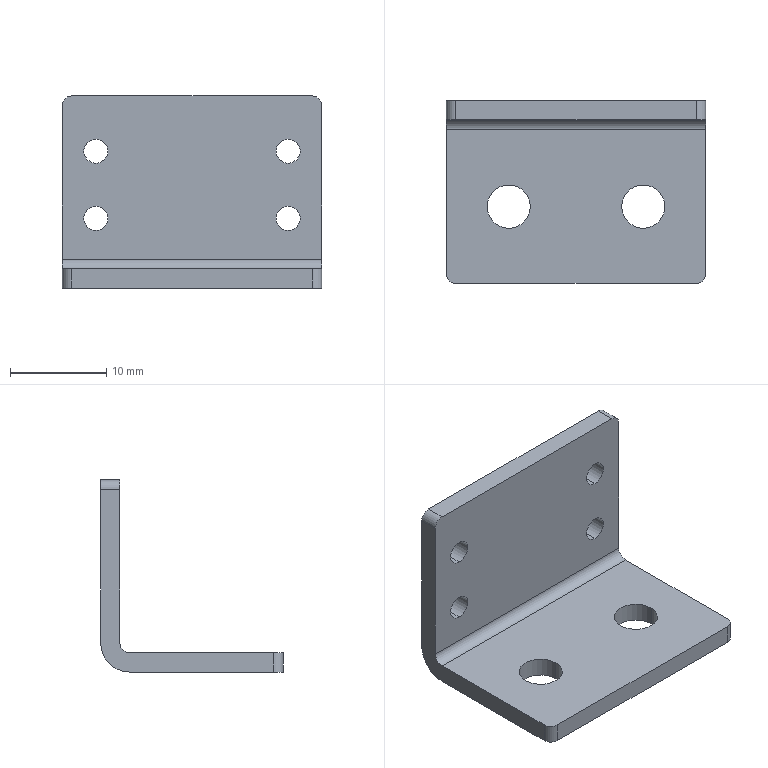Part | SolidWorks | features BaseBody 1 | 1 solid | 26 faces | box 27 x 19 x 20 mm | volume 1847 mm3 | cylinder 18 | plane 8 | commonest cylinder face diameters 2.5 x8 2 x5 4.5 x4 6 x1
STEP:
#1=CARTESIAN_POINT('',(10.,17.,3.));
#2=VERTEX_POINT('',#1);
#3=CARTESIAN_POINT('',(10.,17.,5.5));
#4=VERTEX_POINT('',#3);
#5=CARTESIAN_POINT('',(10.,17.,4.25));
#6=DIRECTION('',(0.,1.,0.));
#7=DIRECTION('',(0.,0.,1.));
#8=AXIS2_PLACEMENT_3D('',#5,#6,#7);
#9=CIRCLE('',#8,1.25);
#10=EDGE_CURVE('',#2,#4,#9,.T.);
#11=ORIENTED_EDGE('',*,*,#10,.F.);
#12=CARTESIAN_POINT('',(10.,19.,3.));
#13=VERTEX_POINT('',#12);
#14=CARTESIAN_POINT('',(10.,19.,3.));
#15=DIRECTION('',(0.,1.,0.));
#16=VECTOR('',#15,1000.);
#17=LINE('',#14,#16);
#18=EDGE_CURVE('',#2,#13,#17,.T.);
#19=ORIENTED_EDGE('',*,*,#18,.T.);
#20=CARTESIAN_POINT('',(10.,19.,5.5));
#21=VERTEX_POINT('',#20);
#22=CARTESIAN_POINT('',(10.,19.,4.25));
#23=DIRECTION('',(0.,-1.,0.));
#24=DIRECTION('',(0.,0.,1.));
#25=AXIS2_PLACEMENT_3D('',#22,#23,#24);
#26=CIRCLE('',#25,1.25);
#27=EDGE_CURVE('',#21,#13,#26,.T.);
#28=ORIENTED_EDGE('',*,*,#27,.F.);
#29=CARTESIAN_POINT('',(10.,19.,5.5));
#30=DIRECTION('',(0.,1.,0.));
#31=VECTOR('',#30,1000.);
#32=LINE('',#29,#31);
#33=EDGE_CURVE('',#4,#21,#32,.T.);
#34=ORIENTED_EDGE('',*,*,#33,.F.);
#35=EDGE_LOOP('',(#11,#19,#28,#34));
#36=FACE_OUTER_BOUND('',#35,.T.);
#37=CARTESIAN_POINT('',(10.,19.,4.25));
#38=DIRECTION('',(0.,1.,0.));
#39=DIRECTION('',(0.,0.,1.));
#40=AXIS2_PLACEMENT_3D('',#37,#38,#39);
#41=CYLINDRICAL_SURFACE('',#40,1.25);
#42=ADVANCED_FACE('',(#36),#41,.F.);
#43=CARTESIAN_POINT('',(10.,17.,-4.));
#44=VERTEX_POINT('',#43);
#45=CARTESIAN_POINT('',(10.,17.,-1.5));
#46=VERTEX_POINT('',#45);
#47=CARTESIAN_POINT('',(10.,17.,-2.75));
#48=DIRECTION('',(0.,1.,0.));
#49=DIRECTION('',(0.,0.,1.));
#50=AXIS2_PLACEMENT_3D('',#47,#48,#49);
#51=CIRCLE('',#50,1.25);
#52=EDGE_CURVE('',#44,#46,#51,.T.);
#53=ORIENTED_EDGE('',*,*,#52,.F.);
#54=CARTESIAN_POINT('',(10.,19.,-4.));
#55=VERTEX_POINT('',#54);
#56=CARTESIAN_POINT('',(10.,19.,-4.));
#57=DIRECTION('',(0.,1.,0.));
#58=VECTOR('',#57,1000.);
#59=LINE('',#56,#58);
#60=EDGE_CURVE('',#44,#55,#59,.T.);
#61=ORIENTED_EDGE('',*,*,#60,.T.);
#62=CARTESIAN_POINT('',(10.,19.,-1.5));
#63=VERTEX_POINT('',#62);
#64=CARTESIAN_POINT('',(10.,19.,-2.75));
#65=DIRECTION('',(0.,-1.,0.));
#66=DIRECTION('',(0.,0.,1.));
#67=AXIS2_PLACEMENT_3D('',#64,#65,#66);
#68=CIRCLE('',#67,1.25);
#69=EDGE_CURVE('',#63,#55,#68,.T.);
#70=ORIENTED_EDGE('',*,*,#69,.F.);
#71=CARTESIAN_POINT('',(10.,19.,-1.5));
#72=DIRECTION('',(0.,1.,0.));
#73=VECTOR('',#72,1000.);
#74=LINE('',#71,#73);
#75=EDGE_CURVE('',#46,#63,#74,.T.);
#76=ORIENTED_EDGE('',*,*,#75,.F.);
#77=EDGE_LOOP('',(#53,#61,#70,#76));
#78=FACE_OUTER_BOUND('',#77,.T.);
#79=CARTESIAN_POINT('',(10.,19.,-2.75));
#80=DIRECTION('',(0.,1.,0.));
#81=DIRECTION('',(0.,0.,1.));
#82=AXIS2_PLACEMENT_3D('',#79,#80,#81);
#83=CYLINDRICAL_SURFACE('',#82,1.25);
#84=ADVANCED_FACE('',(#78),#83,.F.);
#85=CARTESIAN_POINT('',(-10.,17.,-4.));
#86=VERTEX_POINT('',#85);
#87=CARTESIAN_POINT('',(-10.,17.,-1.5));
#88=VERTEX_POINT('',#87);
#89=CARTESIAN_POINT('',(-10.,17.,-2.75));
#90=DIRECTION('',(0.,1.,0.));
#91=DIRECTION('',(0.,0.,1.));
#92=AXIS2_PLACEMENT_3D('',#89,#90,#91);
#93=CIRCLE('',#92,1.25);
#94=EDGE_CURVE('',#86,#88,#93,.T.);
#95=ORIENTED_EDGE('',*,*,#94,.F.);
#96=CARTESIAN_POINT('',(-10.,19.,-4.));
#97=VERTEX_POINT('',#96);
#98=CARTESIAN_POINT('',(-10.,19.,-4.));
#99=DIRECTION('',(0.,1.,0.));
#100=VECTOR('',#99,1000.);
#101=LINE('',#98,#100);
#102=EDGE_CURVE('',#86,#97,#101,.T.);
#103=ORIENTED_EDGE('',*,*,#102,.T.);
#104=CARTESIAN_POINT('',(-10.,19.,-1.5));
#105=VERTEX_POINT('',#104);
#106=CARTESIAN_POINT('',(-10.,19.,-2.75));
#107=DIRECTION('',(0.,-1.,0.));
#108=DIRECTION('',(0.,0.,1.));
#109=AXIS2_PLACEMENT_3D('',#106,#107,#108);
#110=CIRCLE('',#109,1.25);
#111=EDGE_CURVE('',#105,#97,#110,.T.);
#112=ORIENTED_EDGE('',*,*,#111,.F.);
#113=CARTESIAN_POINT('',(-10.,19.,-1.5));
#114=DIRECTION('',(0.,1.,0.));
#115=VECTOR('',#114,1000.);
#116=LINE('',#113,#115);
#117=EDGE_CURVE('',#88,#105,#116,.T.);
#118=ORIENTED_EDGE('',*,*,#117,.F.);
#119=EDGE_LOOP('',(#95,#103,#112,#118));
#120=FACE_OUTER_BOUND('',#119,.T.);
#121=CARTESIAN_POINT('',(-10.,19.,-2.75));
#122=DIRECTION('',(0.,1.,0.));
#123=DIRECTION('',(0.,0.,1.));
#124=AXIS2_PLACEMENT_3D('',#121,#122,#123);
#125=CYLINDRICAL_SURFACE('',#124,1.25);
#126=ADVANCED_FACE('',(#120),#125,.F.);
#127=CARTESIAN_POINT('',(-10.,17.,3.));
#128=VERTEX_POINT('',#127);
#129=CARTESIAN_POINT('',(-10.,17.,5.5));
#130=VERTEX_POINT('',#129);
#131=CARTESIAN_POINT('',(-10.,17.,4.25));
#132=DIRECTION('',(0.,1.,0.));
#133=DIRECTION('',(0.,0.,1.));
#134=AXIS2_PLACEMENT_3D('',#131,#132,#133);
#135=CIRCLE('',#134,1.25);
#136=EDGE_CURVE('',#128,#130,#135,.T.);
#137=ORIENTED_EDGE('',*,*,#136,.F.);
#138=CARTESIAN_POINT('',(-10.,19.,3.));
#139=VERTEX_POINT('',#138);
#140=CARTESIAN_POINT('',(-10.,19.,3.));
#141=DIRECTION('',(0.,1.,0.));
#142=VECTOR('',#141,1000.);
#143=LINE('',#140,#142);
#144=EDGE_CURVE('',#128,#139,#143,.T.);
#145=ORIENTED_EDGE('',*,*,#144,.T.);
#146=CARTESIAN_POINT('',(-10.,19.,5.5));
#147=VERTEX_POINT('',#146);
#148=CARTESIAN_POINT('',(-10.,19.,4.25));
#149=DIRECTION('',(0.,-1.,0.));
#150=DIRECTION('',(0.,0.,1.));
#151=AXIS2_PLACEMENT_3D('',#148,#149,#150);
#152=CIRCLE('',#151,1.25);
#153=EDGE_CURVE('',#147,#139,#152,.T.);
#154=ORIENTED_EDGE('',*,*,#153,.F.);
#155=CARTESIAN_POINT('',(-10.,19.,5.5));
#156=DIRECTION('',(0.,1.,0.));
#157=VECTOR('',#156,1000.);
#158=LINE('',#155,#157);
#159=EDGE_CURVE('',#130,#147,#158,.T.);
#160=ORIENTED_EDGE('',*,*,#159,.F.);
#161=EDGE_LOOP('',(#137,#145,#154,#160));
#162=FACE_OUTER_BOUND('',#161,.T.);
#163=CARTESIAN_POINT('',(-10.,19.,4.25));
#164=DIRECTION('',(0.,1.,0.));
#165=DIRECTION('',(0.,0.,1.));
#166=AXIS2_PLACEMENT_3D('',#163,#164,#165);
#167=CYLINDRICAL_SURFACE('',#166,1.25);
#168=ADVANCED_FACE('',(#162),#167,.F.);
#169=CARTESIAN_POINT('',(9.25,8.,-8.));
#170=VERTEX_POINT('',#169);
#171=CARTESIAN_POINT('',(4.75,8.,-8.));
#172=VERTEX_POINT('',#171);
#173=CARTESIAN_POINT('',(7.,8.,-8.));
#174=DIRECTION('',(0.,0.,-1.));
#175=DIRECTION('',(-1.,0.,0.));
#176=AXIS2_PLACEMENT_3D('',#173,#174,#175);
#177=CIRCLE('',#176,2.25);
#178=EDGE_CURVE('',#170,#172,#177,.T.);
#179=ORIENTED_EDGE('',*,*,#178,.F.);
#180=CARTESIAN_POINT('',(9.25,8.,-10.));
#181=VERTEX_POINT('',#180);
#182=CARTESIAN_POINT('',(9.25,8.,-10.));
#183=DIRECTION('',(0.,0.,-1.));
#184=VECTOR('',#183,1000.);
#185=LINE('',#182,#184);
#186=EDGE_CURVE('',#170,#181,#185,.T.);
#187=ORIENTED_EDGE('',*,*,#186,.T.);
#188=CARTESIAN_POINT('',(4.75,8.,-10.));
#189=VERTEX_POINT('',#188);
#190=CARTESIAN_POINT('',(7.,8.,-10.));
#191=DIRECTION('',(0.,0.,-1.));
#192=DIRECTION('',(-1.,0.,0.));
#193=AXIS2_PLACEMENT_3D('',#190,#191,#192);
#194=CIRCLE('',#193,2.25);
#195=EDGE_CURVE('',#181,#189,#194,.T.);
#196=ORIENTED_EDGE('',*,*,#195,.T.);
#197=CARTESIAN_POINT('',(4.75,8.,-10.));
#198=DIRECTION('',(0.,0.,-1.));
#199=VECTOR('',#198,1000.);
#200=LINE('',#197,#199);
#201=EDGE_CURVE('',#172,#189,#200,.T.);
#202=ORIENTED_EDGE('',*,*,#201,.F.);
#203=EDGE_LOOP('',(#179,#187,#196,#202));
#204=FACE_OUTER_BOUND('',#203,.T.);
#205=CARTESIAN_POINT('',(7.,8.,-10.));
#206=DIRECTION('',(0.,0.,-1.));
#207=DIRECTION('',(-1.,0.,0.));
#208=AXIS2_PLACEMENT_3D('',#205,#206,#207);
#209=CYLINDRICAL_SURFACE('',#208,2.25);
#210=ADVANCED_FACE('',(#204),#209,.F.);
#211=CARTESIAN_POINT('',(-4.75,8.,-8.));
#212=VERTEX_POINT('',#211);
#213=CARTESIAN_POINT('',(-9.25,8.,-8.));
#214=VERTEX_POINT('',#213);
#215=CARTESIAN_POINT('',(-7.,8.,-8.));
#216=DIRECTION('',(0.,0.,-1.));
#217=DIRECTION('',(-1.,0.,0.));
#218=AXIS2_PLACEMENT_3D('',#215,#216,#217);
#219=CIRCLE('',#218,2.25);
#220=EDGE_CURVE('',#212,#214,#219,.T.);
#221=ORIENTED_EDGE('',*,*,#220,.F.);
#222=CARTESIAN_POINT('',(-4.75,8.,-10.));
#223=VERTEX_POINT('',#222);
#224=CARTESIAN_POINT('',(-4.75,8.,-10.));
#225=DIRECTION('',(0.,0.,-1.));
#226=VECTOR('',#225,1000.);
#227=LINE('',#224,#226);
#228=EDGE_CURVE('',#212,#223,#227,.T.);
#229=ORIENTED_EDGE('',*,*,#228,.T.);
#230=CARTESIAN_POINT('',(-9.25,8.,-10.));
#231=VERTEX_POINT('',#230);
#232=CARTESIAN_POINT('',(-7.,8.,-10.));
#233=DIRECTION('',(0.,0.,-1.));
#234=DIRECTION('',(-1.,0.,0.));
#235=AXIS2_PLACEMENT_3D('',#232,#233,#234);
#236=CIRCLE('',#235,2.25);
#237=EDGE_CURVE('',#223,#231,#236,.T.);
#238=ORIENTED_EDGE('',*,*,#237,.T.);
#239=CARTESIAN_POINT('',(-9.25,8.,-10.));
#240=DIRECTION('',(0.,0.,-1.));
#241=VECTOR('',#240,1000.);
#242=LINE('',#239,#241);
#243=EDGE_CURVE('',#214,#231,#242,.T.);
#244=ORIENTED_EDGE('',*,*,#243,.F.);
#245=EDGE_LOOP('',(#221,#229,#238,#244));
#246=FACE_OUTER_BOUND('',#245,.T.);
#247=CARTESIAN_POINT('',(-7.,8.,-10.));
#248=DIRECTION('',(0.,0.,-1.));
#249=DIRECTION('',(-1.,0.,0.));
#250=AXIS2_PLACEMENT_3D('',#247,#248,#249);
#251=CYLINDRICAL_SURFACE('',#250,2.25);
#252=ADVANCED_FACE('',(#246),#251,.F.);
#253=ORIENTED_EDGE('',*,*,#27,.T.);
#254=CARTESIAN_POINT('',(10.,19.,4.25));
#255=DIRECTION('',(0.,-1.,0.));
#256=DIRECTION('',(0.,0.,1.));
#257=AXIS2_PLACEMENT_3D('',#254,#255,#256);
#258=CIRCLE('',#257,1.25);
#259=EDGE_CURVE('',#13,#21,#258,.T.);
#260=ORIENTED_EDGE('',*,*,#259,.T.);
#261=EDGE_LOOP('',(#253,#260));
#262=FACE_BOUND('',#261,.T.);
#263=ORIENTED_EDGE('',*,*,#69,.T.);
#264=CARTESIAN_POINT('',(10.,19.,-2.75));
#265=DIRECTION('',(0.,-1.,0.));
#266=DIRECTION('',(0.,0.,1.));
#267=AXIS2_PLACEMENT_3D('',#264,#265,#266);
#268=CIRCLE('',#267,1.25);
#269=EDGE_CURVE('',#55,#63,#268,.T.);
#270=ORIENTED_EDGE('',*,*,#269,.T.);
#271=EDGE_LOOP('',(#263,#270));
#272=FACE_BOUND('',#271,.T.);
#273=ORIENTED_EDGE('',*,*,#111,.T.);
#274=CARTESIAN_POINT('',(-10.,19.,-2.75));
#275=DIRECTION('',(0.,-1.,0.));
#276=DIRECTION('',(0.,0.,1.));
#277=AXIS2_PLACEMENT_3D('',#274,#275,#276);
#278=CIRCLE('',#277,1.25);
#279=EDGE_CURVE('',#97,#105,#278,.T.);
#280=ORIENTED_EDGE('',*,*,#279,.T.);
#281=EDGE_LOOP('',(#273,#280));
#282=FACE_BOUND('',#281,.T.);
#283=ORIENTED_EDGE('',*,*,#153,.T.);
#284=CARTESIAN_POINT('',(-10.,19.,4.25));
#285=DIRECTION('',(0.,-1.,0.));
#286=DIRECTION('',(0.,0.,1.));
#287=AXIS2_PLACEMENT_3D('',#284,#285,#286);
#288=CIRCLE('',#287,1.25);
#289=EDGE_CURVE('',#139,#147,#288,.T.);
#290=ORIENTED_EDGE('',*,*,#289,.T.);
#291=EDGE_LOOP('',(#283,#290));
#292=FACE_BOUND('',#291,.T.);
#293=CARTESIAN_POINT('',(-13.5,19.,-7.));
#294=VERTEX_POINT('',#293);
#295=CARTESIAN_POINT('',(-13.5,19.,9.));
#296=VERTEX_POINT('',#295);
#297=CARTESIAN_POINT('',(-13.5,19.,0.));
#298=DIRECTION('',(0.,0.,1.));
#299=VECTOR('',#298,1000.);
#300=LINE('',#297,#299);
#301=EDGE_CURVE('',#294,#296,#300,.T.);
#302=ORIENTED_EDGE('',*,*,#301,.T.);
#303=CARTESIAN_POINT('',(-12.5,19.,10.));
#304=VERTEX_POINT('',#303);
#305=CARTESIAN_POINT('',(-12.5,19.,9.));
#306=DIRECTION('',(0.,-1.,0.));
#307=DIRECTION('',(0.,0.,-1.));
#308=AXIS2_PLACEMENT_3D('',#305,#306,#307);
#309=CIRCLE('',#308,1.);
#310=EDGE_CURVE('',#304,#296,#309,.T.);
#311=ORIENTED_EDGE('',*,*,#310,.F.);
#312=CARTESIAN_POINT('',(12.5,19.,10.));
#313=VERTEX_POINT('',#312);
#314=CARTESIAN_POINT('',(0.,19.,10.));
#315=DIRECTION('',(1.,0.,0.));
#316=VECTOR('',#315,1000.);
#317=LINE('',#314,#316);
#318=EDGE_CURVE('',#304,#313,#317,.T.);
#319=ORIENTED_EDGE('',*,*,#318,.T.);
#320=CARTESIAN_POINT('',(13.5,19.,9.));
#321=VERTEX_POINT('',#320);
#322=CARTESIAN_POINT('',(12.5,19.,9.));
#323=DIRECTION('',(0.,-1.,0.));
#324=DIRECTION('',(0.,0.,-1.));
#325=AXIS2_PLACEMENT_3D('',#322,#323,#324);
#326=CIRCLE('',#325,1.);
#327=EDGE_CURVE('',#321,#313,#326,.T.);
#328=ORIENTED_EDGE('',*,*,#327,.F.);
#329=CARTESIAN_POINT('',(13.5,19.,-7.));
#330=VERTEX_POINT('',#329);
#331=CARTESIAN_POINT('',(13.5,19.,0.));
#332=DIRECTION('',(0.,0.,-1.));
#333=VECTOR('',#332,1000.);
#334=LINE('',#331,#333);
#335=EDGE_CURVE('',#321,#330,#334,.T.);
#336=ORIENTED_EDGE('',*,*,#335,.T.);
#337=CARTESIAN_POINT('',(0.,19.,-7.));
#338=DIRECTION('',(-1.,0.,0.));
#339=VECTOR('',#338,1000.);
#340=LINE('',#337,#339);
#341=EDGE_CURVE('',#330,#294,#340,.T.);
#342=ORIENTED_EDGE('',*,*,#341,.T.);
#343=EDGE_LOOP('',(#302,#311,#319,#328,#336,#342));
#344=FACE_OUTER_BOUND('',#343,.T.);
#345=CARTESIAN_POINT('',(0.,19.,0.));
#346=DIRECTION('',(0.,1.,0.));
#347=DIRECTION('',(0.,0.,1.));
#348=AXIS2_PLACEMENT_3D('',#345,#346,#347);
#349=PLANE('',#348);
#350=ADVANCED_FACE('',(#262,#272,#282,#292,#344),#349,.T.);
#351=ORIENTED_EDGE('',*,*,#18,.F.);
#352=CARTESIAN_POINT('',(10.,17.,4.25));
#353=DIRECTION('',(0.,1.,0.));
#354=DIRECTION('',(0.,0.,1.));
#355=AXIS2_PLACEMENT_3D('',#352,#353,#354);
#356=CIRCLE('',#355,1.25);
#357=EDGE_CURVE('',#4,#2,#356,.T.);
#358=ORIENTED_EDGE('',*,*,#357,.F.);
#359=ORIENTED_EDGE('',*,*,#33,.T.);
#360=ORIENTED_EDGE('',*,*,#259,.F.);
#361=EDGE_LOOP('',(#351,#358,#359,#360));
#362=FACE_OUTER_BOUND('',#361,.T.);
#363=CARTESIAN_POINT('',(10.,19.,4.25));
#364=DIRECTION('',(0.,1.,0.));
#365=DIRECTION('',(0.,0.,1.));
#366=AXIS2_PLACEMENT_3D('',#363,#364,#365);
#367=CYLINDRICAL_SURFACE('',#366,1.25);
#368=ADVANCED_FACE('',(#362),#367,.F.);
#369=ORIENTED_EDGE('',*,*,#60,.F.);
#370=CARTESIAN_POINT('',(10.,17.,-2.75));
#371=DIRECTION('',(0.,1.,0.));
#372=DIRECTION('',(0.,0.,1.));
#373=AXIS2_PLACEMENT_3D('',#370,#371,#372);
#374=CIRCLE('',#373,1.25);
#375=EDGE_CURVE('',#46,#44,#374,.T.);
#376=ORIENTED_EDGE('',*,*,#375,.F.);
#377=ORIENTED_EDGE('',*,*,#75,.T.);
#378=ORIENTED_EDGE('',*,*,#269,.F.);
#379=EDGE_LOOP('',(#369,#376,#377,#378));
#380=FACE_OUTER_BOUND('',#379,.T.);
#381=CARTESIAN_POINT('',(10.,19.,-2.75));
#382=DIRECTION('',(0.,1.,0.));
#383=DIRECTION('',(0.,0.,1.));
#384=AXIS2_PLACEMENT_3D('',#381,#382,#383);
#385=CYLINDRICAL_SURFACE('',#384,1.25);
#386=ADVANCED_FACE('',(#380),#385,.F.);
#387=ORIENTED_EDGE('',*,*,#102,.F.);
#388=CARTESIAN_POINT('',(-10.,17.,-2.75));
#389=DIRECTION('',(0.,1.,0.));
#390=DIRECTION('',(0.,0.,1.));
#391=AXIS2_PLACEMENT_3D('',#388,#389,#390);
#392=CIRCLE('',#391,1.25);
#393=EDGE_CURVE('',#88,#86,#392,.T.);
#394=ORIENTED_EDGE('',*,*,#393,.F.);
#395=ORIENTED_EDGE('',*,*,#117,.T.);
#396=ORIENTED_EDGE('',*,*,#279,.F.);
#397=EDGE_LOOP('',(#387,#394,#395,#396));
#398=FACE_OUTER_BOUND('',#397,.T.);
#399=CARTESIAN_POINT('',(-10.,19.,-2.75));
#400=DIRECTION('',(0.,1.,0.));
#401=DIRECTION('',(0.,0.,1.));
#402=AXIS2_PLACEMENT_3D('',#399,#400,#401);
#403=CYLINDRICAL_SURFACE('',#402,1.25);
#404=ADVANCED_FACE('',(#398),#403,.F.);
#405=ORIENTED_EDGE('',*,*,#144,.F.);
#406=CARTESIAN_POINT('',(-10.,17.,4.25));
#407=DIRECTION('',(0.,1.,0.));
#408=DIRECTION('',(0.,0.,1.));
#409=AXIS2_PLACEMENT_3D('',#406,#407,#408);
#410=CIRCLE('',#409,1.25);
#411=EDGE_CURVE('',#130,#128,#410,.T.);
#412=ORIENTED_EDGE('',*,*,#411,.F.);
#413=ORIENTED_EDGE('',*,*,#159,.T.);
#414=ORIENTED_EDGE('',*,*,#289,.F.);
#415=EDGE_LOOP('',(#405,#412,#413,#414));
#416=FACE_OUTER_BOUND('',#415,.T.);
#417=CARTESIAN_POINT('',(-10.,19.,4.25));
#418=DIRECTION('',(0.,1.,0.));
#419=DIRECTION('',(0.,0.,1.));
#420=AXIS2_PLACEMENT_3D('',#417,#418,#419);
#421=CYLINDRICAL_SURFACE('',#420,1.25);
#422=ADVANCED_FACE('',(#416),#421,.F.);
#423=CARTESIAN_POINT('',(-13.5,17.,9.));
#424=VERTEX_POINT('',#423);
#425=CARTESIAN_POINT('',(-13.5,17.,-7.));
#426=VERTEX_POINT('',#425);
#427=CARTESIAN_POINT('',(-13.5,17.,-10.));
#428=DIRECTION('',(0.,0.,-1.));
#429=VECTOR('',#428,1000.);
#430=LINE('',#427,#429);
#431=EDGE_CURVE('',#424,#426,#430,.T.);
#432=ORIENTED_EDGE('',*,*,#431,.F.);
#433=CARTESIAN_POINT('',(-13.5,19.,9.));
#434=DIRECTION('',(0.,-1.,0.));
#435=VECTOR('',#434,1000.);
#436=LINE('',#433,#435);
#437=EDGE_CURVE('',#296,#424,#436,.T.);
#438=ORIENTED_EDGE('',*,*,#437,.F.);
#439=ORIENTED_EDGE('',*,*,#301,.F.);
#440=CARTESIAN_POINT('',(-13.5,16.,-10.));
#441=VERTEX_POINT('',#440);
#442=CARTESIAN_POINT('',(-13.5,16.,-7.));
#443=DIRECTION('',(1.,0.,0.));
#444=DIRECTION('',(0.,0.,-1.));
#445=AXIS2_PLACEMENT_3D('',#442,#443,#444);
#446=CIRCLE('',#445,3.);
#447=EDGE_CURVE('',#441,#294,#446,.T.);
#448=ORIENTED_EDGE('',*,*,#447,.F.);
#449=CARTESIAN_POINT('',(-13.5,1.,-10.));
#450=VERTEX_POINT('',#449);
#451=CARTESIAN_POINT('',(-13.5,19.,-10.));
#452=DIRECTION('',(0.,1.,0.));
#453=VECTOR('',#452,1000.);
#454=LINE('',#451,#453);
#455=EDGE_CURVE('',#450,#441,#454,.T.);
#456=ORIENTED_EDGE('',*,*,#455,.F.);
#457=CARTESIAN_POINT('',(-13.5,1.,-8.));
#458=VERTEX_POINT('',#457);
#459=CARTESIAN_POINT('',(-13.5,1.,-10.));
#460=DIRECTION('',(0.,0.,-1.));
#461=VECTOR('',#460,1000.);
#462=LINE('',#459,#461);
#463=EDGE_CURVE('',#458,#450,#462,.T.);
#464=ORIENTED_EDGE('',*,*,#463,.F.);
#465=CARTESIAN_POINT('',(-13.5,16.,-8.));
#466=VERTEX_POINT('',#465);
#467=CARTESIAN_POINT('',(-13.5,19.,-8.));
#468=DIRECTION('',(0.,-1.,0.));
#469=VECTOR('',#468,1000.);
#470=LINE('',#467,#469);
#471=EDGE_CURVE('',#466,#458,#470,.T.);
#472=ORIENTED_EDGE('',*,*,#471,.F.);
#473=CARTESIAN_POINT('',(-13.5,16.,-7.));
#474=DIRECTION('',(1.,0.,0.));
#475=DIRECTION('',(0.,0.,1.));
#476=AXIS2_PLACEMENT_3D('',#473,#474,#475);
#477=CIRCLE('',#476,1.);
#478=EDGE_CURVE('',#466,#426,#477,.T.);
#479=ORIENTED_EDGE('',*,*,#478,.T.);
#480=EDGE_LOOP('',(#432,#438,#439,#448,#456,#464,#472,#479));
#481=FACE_OUTER_BOUND('',#480,.T.);
#482=CARTESIAN_POINT('',(-13.5,19.,-10.));
#483=DIRECTION('',(1.,0.,0.));
#484=DIRECTION('',(0.,0.,-1.));
#485=AXIS2_PLACEMENT_3D('',#482,#483,#484);
#486=PLANE('',#485);
#487=ADVANCED_FACE('',(#481),#486,.F.);
#488=CARTESIAN_POINT('',(13.5,16.,-10.));
#489=VERTEX_POINT('',#488);
#490=CARTESIAN_POINT('',(13.5,16.,-7.));
#491=DIRECTION('',(-1.,0.,0.));
#492=DIRECTION('',(0.,0.,-1.));
#493=AXIS2_PLACEMENT_3D('',#490,#491,#492);
#494=CIRCLE('',#493,3.);
#495=EDGE_CURVE('',#330,#489,#494,.T.);
#496=ORIENTED_EDGE('',*,*,#495,.T.);
#497=CARTESIAN_POINT('',(0.,16.,-10.));
#498=DIRECTION('',(-1.,0.,0.));
#499=VECTOR('',#498,1000.);
#500=LINE('',#497,#499);
#501=EDGE_CURVE('',#489,#441,#500,.T.);
#502=ORIENTED_EDGE('',*,*,#501,.T.);
#503=ORIENTED_EDGE('',*,*,#447,.T.);
#504=ORIENTED_EDGE('',*,*,#341,.F.);
#505=EDGE_LOOP('',(#496,#502,#503,#504));
#506=FACE_OUTER_BOUND('',#505,.T.);
#507=CARTESIAN_POINT('',(0.,16.,-7.));
#508=DIRECTION('',(1.,0.,0.));
#509=DIRECTION('',(0.,0.,-1.));
#510=AXIS2_PLACEMENT_3D('',#507,#508,#509);
#511=CYLINDRICAL_SURFACE('',#510,3.);
#512=ADVANCED_FACE('',(#506),#511,.T.);
#513=ORIENTED_EDGE('',*,*,#335,.F.);
#514=CARTESIAN_POINT('',(13.5,17.,9.));
#515=VERTEX_POINT('',#514);
#516=CARTESIAN_POINT('',(13.5,19.,9.));
#517=DIRECTION('',(0.,1.,0.));
#518=VECTOR('',#517,1000.);
#519=LINE('',#516,#518);
#520=EDGE_CURVE('',#515,#321,#519,.T.);
#521=ORIENTED_EDGE('',*,*,#520,.F.);
#522=CARTESIAN_POINT('',(13.5,17.,-7.));
#523=VERTEX_POINT('',#522);
#524=CARTESIAN_POINT('',(13.5,17.,-10.));
#525=DIRECTION('',(0.,0.,1.));
#526=VECTOR('',#525,1000.);
#527=LINE('',#524,#526);
#528=EDGE_CURVE('',#523,#515,#527,.T.);
#529=ORIENTED_EDGE('',*,*,#528,.F.);
#530=CARTESIAN_POINT('',(13.5,16.,-8.));
#531=VERTEX_POINT('',#530);
#532=CARTESIAN_POINT('',(13.5,16.,-7.));
#533=DIRECTION('',(-1.,0.,0.));
#534=DIRECTION('',(0.,0.,1.));
#535=AXIS2_PLACEMENT_3D('',#532,#533,#534);
#536=CIRCLE('',#535,1.);
#537=EDGE_CURVE('',#523,#531,#536,.T.);
#538=ORIENTED_EDGE('',*,*,#537,.T.);
#539=CARTESIAN_POINT('',(13.5,1.,-8.));
#540=VERTEX_POINT('',#539);
#541=CARTESIAN_POINT('',(13.5,19.,-8.));
#542=DIRECTION('',(0.,1.,0.));
#543=VECTOR('',#542,1000.);
#544=LINE('',#541,#543);
#545=EDGE_CURVE('',#540,#531,#544,.T.);
#546=ORIENTED_EDGE('',*,*,#545,.F.);
#547=CARTESIAN_POINT('',(13.5,1.,-10.));
#548=VERTEX_POINT('',#547);
#549=CARTESIAN_POINT('',(13.5,1.,-10.));
#550=DIRECTION('',(0.,0.,1.));
#551=VECTOR('',#550,1000.);
#552=LINE('',#549,#551);
#553=EDGE_CURVE('',#548,#540,#552,.T.);
#554=ORIENTED_EDGE('',*,*,#553,.F.);
#555=CARTESIAN_POINT('',(13.5,19.,-10.));
#556=DIRECTION('',(0.,-1.,0.));
#557=VECTOR('',#556,1000.);
#558=LINE('',#555,#557);
#559=EDGE_CURVE('',#489,#548,#558,.T.);
#560=ORIENTED_EDGE('',*,*,#559,.F.);
#561=ORIENTED_EDGE('',*,*,#495,.F.);
#562=EDGE_LOOP('',(#513,#521,#529,#538,#546,#554,#560,#561));
#563=FACE_OUTER_BOUND('',#562,.T.);
#564=CARTESIAN_POINT('',(13.5,19.,-10.));
#565=DIRECTION('',(-1.,0.,0.));
#566=DIRECTION('',(0.,0.,1.));
#567=AXIS2_PLACEMENT_3D('',#564,#565,#566);
#568=PLANE('',#567);
#569=ADVANCED_FACE('',(#563),#568,.F.);
#570=CARTESIAN_POINT('',(12.5,17.,10.));
#571=VERTEX_POINT('',#570);
#572=CARTESIAN_POINT('',(-12.5,17.,10.));
#573=VERTEX_POINT('',#572);
#574=CARTESIAN_POINT('',(-13.5,17.,10.));
#575=DIRECTION('',(-1.,0.,0.));
#576=VECTOR('',#575,1000.);
#577=LINE('',#574,#576);
#578=EDGE_CURVE('',#571,#573,#577,.T.);
#579=ORIENTED_EDGE('',*,*,#578,.F.);
#580=CARTESIAN_POINT('',(12.5,19.,10.));
#581=DIRECTION('',(0.,-1.,0.));
#582=VECTOR('',#581,1000.);
#583=LINE('',#580,#582);
#584=EDGE_CURVE('',#313,#571,#583,.T.);
#585=ORIENTED_EDGE('',*,*,#584,.F.);
#586=ORIENTED_EDGE('',*,*,#318,.F.);
#587=CARTESIAN_POINT('',(-12.5,19.,10.));
#588=DIRECTION('',(0.,1.,0.));
#589=VECTOR('',#588,1000.);
#590=LINE('',#587,#589);
#591=EDGE_CURVE('',#573,#304,#590,.T.);
#592=ORIENTED_EDGE('',*,*,#591,.F.);
#593=EDGE_LOOP('',(#579,#585,#586,#592));
#594=FACE_OUTER_BOUND('',#593,.T.);
#595=CARTESIAN_POINT('',(-13.5,19.,10.));
#596=DIRECTION('',(0.,0.,-1.));
#597=DIRECTION('',(-1.,0.,0.));
#598=AXIS2_PLACEMENT_3D('',#595,#596,#597);
#599=PLANE('',#598);
#600=ADVANCED_FACE('',(#594),#599,.F.);
#601=ORIENTED_EDGE('',*,*,#357,.T.);
#602=ORIENTED_EDGE('',*,*,#10,.T.);
#603=EDGE_LOOP('',(#601,#602));
#604=FACE_BOUND('',#603,.T.);
#605=ORIENTED_EDGE('',*,*,#375,.T.);
#606=ORIENTED_EDGE('',*,*,#52,.T.);
#607=EDGE_LOOP('',(#605,#606));
#608=FACE_BOUND('',#607,.T.);
#609=ORIENTED_EDGE('',*,*,#393,.T.);
#610=ORIENTED_EDGE('',*,*,#94,.T.);
#611=EDGE_LOOP('',(#609,#610));
#612=FACE_BOUND('',#611,.T.);
#613=ORIENTED_EDGE('',*,*,#411,.T.);
#614=ORIENTED_EDGE('',*,*,#136,.T.);
#615=EDGE_LOOP('',(#613,#614));
#616=FACE_BOUND('',#615,.T.);
#617=ORIENTED_EDGE('',*,*,#431,.T.);
#618=CARTESIAN_POINT('',(0.,17.,-7.));
#619=DIRECTION('',(-1.,0.,0.));
#620=VECTOR('',#619,1000.);
#621=LINE('',#618,#620);
#622=EDGE_CURVE('',#523,#426,#621,.T.);
#623=ORIENTED_EDGE('',*,*,#622,.F.);
#624=ORIENTED_EDGE('',*,*,#528,.T.);
#625=CARTESIAN_POINT('',(12.5,17.,9.));
#626=DIRECTION('',(0.,1.,0.));
#627=DIRECTION('',(0.,0.,-1.));
#628=AXIS2_PLACEMENT_3D('',#625,#626,#627);
#629=CIRCLE('',#628,1.);
#630=EDGE_CURVE('',#571,#515,#629,.T.);
#631=ORIENTED_EDGE('',*,*,#630,.F.);
#632=ORIENTED_EDGE('',*,*,#578,.T.);
#633=CARTESIAN_POINT('',(-12.5,17.,9.));
#634=DIRECTION('',(0.,1.,0.));
#635=DIRECTION('',(0.,0.,-1.));
#636=AXIS2_PLACEMENT_3D('',#633,#634,#635);
#637=CIRCLE('',#636,1.);
#638=EDGE_CURVE('',#424,#573,#637,.T.);
#639=ORIENTED_EDGE('',*,*,#638,.F.);
#640=EDGE_LOOP('',(#617,#623,#624,#631,#632,#639));
#641=FACE_OUTER_BOUND('',#640,.T.);
#642=CARTESIAN_POINT('',(0.,17.,0.));
#643=DIRECTION('',(0.,1.,0.));
#644=DIRECTION('',(0.,0.,1.));
#645=AXIS2_PLACEMENT_3D('',#642,#643,#644);
#646=PLANE('',#645);
#647=ADVANCED_FACE('',(#604,#608,#612,#616,#641),#646,.F.);
#648=ORIENTED_EDGE('',*,*,#310,.T.);
#649=ORIENTED_EDGE('',*,*,#437,.T.);
#650=ORIENTED_EDGE('',*,*,#638,.T.);
#651=ORIENTED_EDGE('',*,*,#591,.T.);
#652=EDGE_LOOP('',(#648,#649,#650,#651));
#653=FACE_OUTER_BOUND('',#652,.T.);
#654=CARTESIAN_POINT('',(-12.5,19.,9.));
#655=DIRECTION('',(0.,-1.,0.));
#656=DIRECTION('',(0.,0.,-1.));
#657=AXIS2_PLACEMENT_3D('',#654,#655,#656);
#658=CYLINDRICAL_SURFACE('',#657,1.);
#659=ADVANCED_FACE('',(#653),#658,.T.);
#660=CARTESIAN_POINT('',(7.,8.,-10.));
#661=DIRECTION('',(0.,0.,-1.));
#662=DIRECTION('',(-1.,0.,0.));
#663=AXIS2_PLACEMENT_3D('',#660,#661,#662);
#664=CIRCLE('',#663,2.25);
#665=EDGE_CURVE('',#189,#181,#664,.T.);
#666=ORIENTED_EDGE('',*,*,#665,.F.);
#667=ORIENTED_EDGE('',*,*,#195,.F.);
#668=EDGE_LOOP('',(#666,#667));
#669=FACE_BOUND('',#668,.T.);
#670=CARTESIAN_POINT('',(-7.,8.,-10.));
#671=DIRECTION('',(0.,0.,-1.));
#672=DIRECTION('',(-1.,0.,0.));
#673=AXIS2_PLACEMENT_3D('',#670,#671,#672);
#674=CIRCLE('',#673,2.25);
#675=EDGE_CURVE('',#231,#223,#674,.T.);
#676=ORIENTED_EDGE('',*,*,#675,.F.);
#677=ORIENTED_EDGE('',*,*,#237,.F.);
#678=EDGE_LOOP('',(#676,#677));
#679=FACE_BOUND('',#678,.T.);
#680=ORIENTED_EDGE('',*,*,#559,.T.);
#681=CARTESIAN_POINT('',(12.5,0.,-10.));
#682=VERTEX_POINT('',#681);
#683=CARTESIAN_POINT('',(12.5,1.,-10.));
#684=DIRECTION('',(0.,0.,1.));
#685=DIRECTION('',(-1.,0.,0.));
#686=AXIS2_PLACEMENT_3D('',#683,#684,#685);
#687=CIRCLE('',#686,1.);
#688=EDGE_CURVE('',#682,#548,#687,.T.);
#689=ORIENTED_EDGE('',*,*,#688,.F.);
#690=CARTESIAN_POINT('',(-12.5,0.,-10.));
#691=VERTEX_POINT('',#690);
#692=CARTESIAN_POINT('',(-13.5,0.,-10.));
#693=DIRECTION('',(1.,0.,0.));
#694=VECTOR('',#693,1000.);
#695=LINE('',#692,#694);
#696=EDGE_CURVE('',#691,#682,#695,.T.);
#697=ORIENTED_EDGE('',*,*,#696,.F.);
#698=CARTESIAN_POINT('',(-12.5,1.,-10.));
#699=DIRECTION('',(0.,0.,1.));
#700=DIRECTION('',(1.,0.,0.));
#701=AXIS2_PLACEMENT_3D('',#698,#699,#700);
#702=CIRCLE('',#701,1.);
#703=EDGE_CURVE('',#450,#691,#702,.T.);
#704=ORIENTED_EDGE('',*,*,#703,.F.);
#705=ORIENTED_EDGE('',*,*,#455,.T.);
#706=ORIENTED_EDGE('',*,*,#501,.F.);
#707=EDGE_LOOP('',(#680,#689,#697,#704,#705,#706));
#708=FACE_OUTER_BOUND('',#707,.T.);
#709=CARTESIAN_POINT('',(-13.5,19.,-10.));
#710=DIRECTION('',(0.,0.,1.));
#711=DIRECTION('',(1.,0.,0.));
#712=AXIS2_PLACEMENT_3D('',#709,#710,#711);
#713=PLANE('',#712);
#714=ADVANCED_FACE('',(#669,#679,#708),#713,.F.);
#715=ORIENTED_EDGE('',*,*,#703,.T.);
#716=CARTESIAN_POINT('',(-12.5,0.,-8.));
#717=VERTEX_POINT('',#716);
#718=CARTESIAN_POINT('',(-12.5,0.,-10.));
#719=DIRECTION('',(0.,0.,1.));
#720=VECTOR('',#719,1000.);
#721=LINE('',#718,#720);
#722=EDGE_CURVE('',#691,#717,#721,.T.);
#723=ORIENTED_EDGE('',*,*,#722,.T.);
#724=CARTESIAN_POINT('',(-12.5,1.,-8.));
#725=DIRECTION('',(0.,0.,-1.));
#726=DIRECTION('',(1.,0.,0.));
#727=AXIS2_PLACEMENT_3D('',#724,#725,#726);
#728=CIRCLE('',#727,1.);
#729=EDGE_CURVE('',#717,#458,#728,.T.);
#730=ORIENTED_EDGE('',*,*,#729,.T.);
#731=ORIENTED_EDGE('',*,*,#463,.T.);
#732=EDGE_LOOP('',(#715,#723,#730,#731));
#733=FACE_OUTER_BOUND('',#732,.T.);
#734=CARTESIAN_POINT('',(-12.5,1.,-10.));
#735=DIRECTION('',(0.,0.,1.));
#736=DIRECTION('',(1.,0.,0.));
#737=AXIS2_PLACEMENT_3D('',#734,#735,#736);
#738=CYLINDRICAL_SURFACE('',#737,1.);
#739=ADVANCED_FACE('',(#733),#738,.T.);
#740=CARTESIAN_POINT('',(7.,8.,-8.));
#741=DIRECTION('',(0.,0.,-1.));
#742=DIRECTION('',(-1.,0.,0.));
#743=AXIS2_PLACEMENT_3D('',#740,#741,#742);
#744=CIRCLE('',#743,2.25);
#745=EDGE_CURVE('',#172,#170,#744,.T.);
#746=ORIENTED_EDGE('',*,*,#745,.T.);
#747=ORIENTED_EDGE('',*,*,#178,.T.);
#748=EDGE_LOOP('',(#746,#747));
#749=FACE_BOUND('',#748,.T.);
#750=CARTESIAN_POINT('',(-7.,8.,-8.));
#751=DIRECTION('',(0.,0.,-1.));
#752=DIRECTION('',(-1.,0.,0.));
#753=AXIS2_PLACEMENT_3D('',#750,#751,#752);
#754=CIRCLE('',#753,2.25);
#755=EDGE_CURVE('',#214,#212,#754,.T.);
#756=ORIENTED_EDGE('',*,*,#755,.T.);
#757=ORIENTED_EDGE('',*,*,#220,.T.);
#758=EDGE_LOOP('',(#756,#757));
#759=FACE_BOUND('',#758,.T.);
#760=ORIENTED_EDGE('',*,*,#545,.T.);
#761=CARTESIAN_POINT('',(-13.5,16.,-8.));
#762=DIRECTION('',(-1.,0.,0.));
#763=VECTOR('',#762,1000.);
#764=LINE('',#761,#763);
#765=EDGE_CURVE('',#531,#466,#764,.T.);
#766=ORIENTED_EDGE('',*,*,#765,.T.);
#767=ORIENTED_EDGE('',*,*,#471,.T.);
#768=ORIENTED_EDGE('',*,*,#729,.F.);
#769=CARTESIAN_POINT('',(12.5,0.,-8.));
#770=VERTEX_POINT('',#769);
#771=CARTESIAN_POINT('',(-13.5,0.,-8.));
#772=DIRECTION('',(1.,0.,0.));
#773=VECTOR('',#772,1000.);
#774=LINE('',#771,#773);
#775=EDGE_CURVE('',#717,#770,#774,.T.);
#776=ORIENTED_EDGE('',*,*,#775,.T.);
#777=CARTESIAN_POINT('',(12.5,1.,-8.));
#778=DIRECTION('',(0.,0.,1.));
#779=DIRECTION('',(-1.,0.,0.));
#780=AXIS2_PLACEMENT_3D('',#777,#778,#779);
#781=CIRCLE('',#780,1.);
#782=EDGE_CURVE('',#770,#540,#781,.T.);
#783=ORIENTED_EDGE('',*,*,#782,.T.);
#784=EDGE_LOOP('',(#760,#766,#767,#768,#776,#783));
#785=FACE_OUTER_BOUND('',#784,.T.);
#786=CARTESIAN_POINT('',(-13.5,19.,-8.));
#787=DIRECTION('',(0.,0.,1.));
#788=DIRECTION('',(1.,0.,0.));
#789=AXIS2_PLACEMENT_3D('',#786,#787,#788);
#790=PLANE('',#789);
#791=ADVANCED_FACE('',(#749,#759,#785),#790,.T.);
#792=ORIENTED_EDGE('',*,*,#327,.T.);
#793=ORIENTED_EDGE('',*,*,#584,.T.);
#794=ORIENTED_EDGE('',*,*,#630,.T.);
#795=ORIENTED_EDGE('',*,*,#520,.T.);
#796=EDGE_LOOP('',(#792,#793,#794,#795));
#797=FACE_OUTER_BOUND('',#796,.T.);
#798=CARTESIAN_POINT('',(12.5,19.,9.));
#799=DIRECTION('',(0.,-1.,0.));
#800=DIRECTION('',(0.,0.,-1.));
#801=AXIS2_PLACEMENT_3D('',#798,#799,#800);
#802=CYLINDRICAL_SURFACE('',#801,1.);
#803=ADVANCED_FACE('',(#797),#802,.T.);
#804=ORIENTED_EDGE('',*,*,#782,.F.);
#805=CARTESIAN_POINT('',(12.5,0.,-10.));
#806=DIRECTION('',(0.,0.,-1.));
#807=VECTOR('',#806,1000.);
#808=LINE('',#805,#807);
#809=EDGE_CURVE('',#770,#682,#808,.T.);
#810=ORIENTED_EDGE('',*,*,#809,.T.);
#811=ORIENTED_EDGE('',*,*,#688,.T.);
#812=ORIENTED_EDGE('',*,*,#553,.T.);
#813=EDGE_LOOP('',(#804,#810,#811,#812));
#814=FACE_OUTER_BOUND('',#813,.T.);
#815=CARTESIAN_POINT('',(12.5,1.,-10.));
#816=DIRECTION('',(0.,0.,-1.));
#817=DIRECTION('',(-1.,0.,0.));
#818=AXIS2_PLACEMENT_3D('',#815,#816,#817);
#819=CYLINDRICAL_SURFACE('',#818,1.);
#820=ADVANCED_FACE('',(#814),#819,.T.);
#821=ORIENTED_EDGE('',*,*,#537,.F.);
#822=ORIENTED_EDGE('',*,*,#622,.T.);
#823=ORIENTED_EDGE('',*,*,#478,.F.);
#824=ORIENTED_EDGE('',*,*,#765,.F.);
#825=EDGE_LOOP('',(#821,#822,#823,#824));
#826=FACE_OUTER_BOUND('',#825,.T.);
#827=CARTESIAN_POINT('',(-13.5,16.,-7.));
#828=DIRECTION('',(-1.,0.,0.));
#829=DIRECTION('',(0.,0.,1.));
#830=AXIS2_PLACEMENT_3D('',#827,#828,#829);
#831=CYLINDRICAL_SURFACE('',#830,1.);
#832=ADVANCED_FACE('',(#826),#831,.F.);
#833=ORIENTED_EDGE('',*,*,#186,.F.);
#834=ORIENTED_EDGE('',*,*,#745,.F.);
#835=ORIENTED_EDGE('',*,*,#201,.T.);
#836=ORIENTED_EDGE('',*,*,#665,.T.);
#837=EDGE_LOOP('',(#833,#834,#835,#836));
#838=FACE_OUTER_BOUND('',#837,.T.);
#839=CARTESIAN_POINT('',(7.,8.,-10.));
#840=DIRECTION('',(0.,0.,-1.));
#841=DIRECTION('',(-1.,0.,0.));
#842=AXIS2_PLACEMENT_3D('',#839,#840,#841);
#843=CYLINDRICAL_SURFACE('',#842,2.25);
#844=ADVANCED_FACE('',(#838),#843,.F.);
#845=ORIENTED_EDGE('',*,*,#228,.F.);
#846=ORIENTED_EDGE('',*,*,#755,.F.);
#847=ORIENTED_EDGE('',*,*,#243,.T.);
#848=ORIENTED_EDGE('',*,*,#675,.T.);
#849=EDGE_LOOP('',(#845,#846,#847,#848));
#850=FACE_OUTER_BOUND('',#849,.T.);
#851=CARTESIAN_POINT('',(-7.,8.,-10.));
#852=DIRECTION('',(0.,0.,-1.));
#853=DIRECTION('',(-1.,0.,0.));
#854=AXIS2_PLACEMENT_3D('',#851,#852,#853);
#855=CYLINDRICAL_SURFACE('',#854,2.25);
#856=ADVANCED_FACE('',(#850),#855,.F.);
#857=ORIENTED_EDGE('',*,*,#775,.F.);
#858=ORIENTED_EDGE('',*,*,#722,.F.);
#859=ORIENTED_EDGE('',*,*,#696,.T.);
#860=ORIENTED_EDGE('',*,*,#809,.F.);
#861=EDGE_LOOP('',(#857,#858,#859,#860));
#862=FACE_OUTER_BOUND('',#861,.T.);
#863=CARTESIAN_POINT('',(0.,0.,0.));
#864=DIRECTION('',(0.,1.,0.));
#865=DIRECTION('',(0.,0.,1.));
#866=AXIS2_PLACEMENT_3D('',#863,#864,#865);
#867=PLANE('',#866);
#868=ADVANCED_FACE('',(#862),#867,.F.);
#869=CLOSED_SHELL('',(#42,#84,#126,#168,#210,#252,#350,#368,#386,#404,#422,#487,#512,#569,#600,#647,#659,#714,#739,#791,#803,#820,#832,#844,#856,#868));
#870=MANIFOLD_SOLID_BREP('',#869);
#871=CARTESIAN_POINT('',(0.,0.,0.));
#872=DIRECTION('',(0.,0.,1.));
#873=DIRECTION('',(1.,0.,0.));
#874=AXIS2_PLACEMENT_3D('',#871,#872,#873);
#875=(LENGTH_UNIT()NAMED_UNIT(*)SI_UNIT(.MILLI.,.METRE.));
#876=UNCERTAINTY_MEASURE_WITH_UNIT(LENGTH_MEASURE(0.00001),#875,'','');
#877=(NAMED_UNIT(*)PLANE_ANGLE_UNIT()SI_UNIT($,.RADIAN.));
#878=(NAMED_UNIT(*)SI_UNIT($,.STERADIAN.)SOLID_ANGLE_UNIT());
#879=(GEOMETRIC_REPRESENTATION_CONTEXT(3)GLOBAL_UNCERTAINTY_ASSIGNED_CONTEXT((#876))GLOBAL_UNIT_ASSIGNED_CONTEXT((#875,#877,#878))REPRESENTATION_CONTEXT('',''));
#880=ADVANCED_BREP_SHAPE_REPRESENTATION('',(#870,#874),#879);